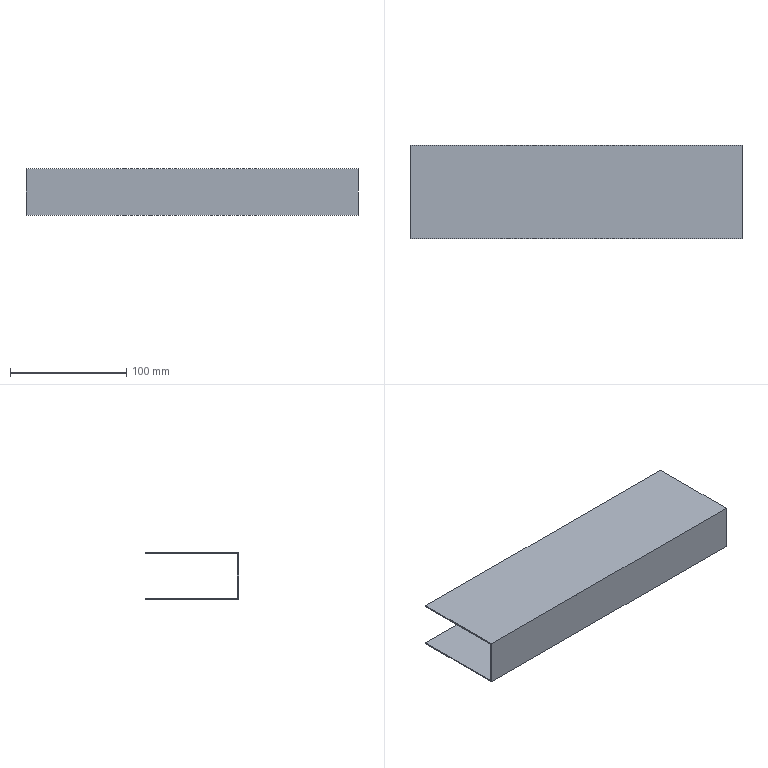Part | SolidWorks | features BaseBody 1 | 1 solid | 10 faces | box 285 x 80 x 40 mm | volume 56430 mm3 | plane 10
STEP:
#1=CARTESIAN_POINT('',(0.,1.,19.));
#2=VERTEX_POINT('',#1);
#3=CARTESIAN_POINT('',(0.,80.,19.));
#4=VERTEX_POINT('',#3);
#5=CARTESIAN_POINT('',(0.,0.,19.));
#6=DIRECTION('',(0.,1.,0.));
#7=VECTOR('',#6,1000.);
#8=LINE('',#5,#7);
#9=EDGE_CURVE('',#2,#4,#8,.T.);
#10=ORIENTED_EDGE('',*,*,#9,.F.);
#11=CARTESIAN_POINT('',(0.,1.,-19.));
#12=VERTEX_POINT('',#11);
#13=CARTESIAN_POINT('',(0.,1.,20.));
#14=DIRECTION('',(0.,0.,1.));
#15=VECTOR('',#14,1000.);
#16=LINE('',#13,#15);
#17=EDGE_CURVE('',#12,#2,#16,.T.);
#18=ORIENTED_EDGE('',*,*,#17,.F.);
#19=CARTESIAN_POINT('',(0.,80.,-19.));
#20=VERTEX_POINT('',#19);
#21=CARTESIAN_POINT('',(0.,0.,-19.));
#22=DIRECTION('',(0.,-1.,0.));
#23=VECTOR('',#22,1000.);
#24=LINE('',#21,#23);
#25=EDGE_CURVE('',#20,#12,#24,.T.);
#26=ORIENTED_EDGE('',*,*,#25,.F.);
#27=CARTESIAN_POINT('',(0.,80.,-20.));
#28=VERTEX_POINT('',#27);
#29=CARTESIAN_POINT('',(0.,80.,-19.));
#30=DIRECTION('',(0.,0.,-1.));
#31=VECTOR('',#30,1000.);
#32=LINE('',#29,#31);
#33=EDGE_CURVE('',#20,#28,#32,.T.);
#34=ORIENTED_EDGE('',*,*,#33,.T.);
#35=CARTESIAN_POINT('',(0.,0.,-20.));
#36=VERTEX_POINT('',#35);
#37=CARTESIAN_POINT('',(0.,0.,-20.));
#38=DIRECTION('',(0.,-1.,0.));
#39=VECTOR('',#38,1000.);
#40=LINE('',#37,#39);
#41=EDGE_CURVE('',#28,#36,#40,.T.);
#42=ORIENTED_EDGE('',*,*,#41,.T.);
#43=CARTESIAN_POINT('',(0.,0.,20.));
#44=VERTEX_POINT('',#43);
#45=CARTESIAN_POINT('',(0.,0.,20.));
#46=DIRECTION('',(0.,0.,1.));
#47=VECTOR('',#46,1000.);
#48=LINE('',#45,#47);
#49=EDGE_CURVE('',#36,#44,#48,.T.);
#50=ORIENTED_EDGE('',*,*,#49,.T.);
#51=CARTESIAN_POINT('',(0.,80.,20.));
#52=VERTEX_POINT('',#51);
#53=CARTESIAN_POINT('',(0.,0.,20.));
#54=DIRECTION('',(0.,1.,0.));
#55=VECTOR('',#54,1000.);
#56=LINE('',#53,#55);
#57=EDGE_CURVE('',#44,#52,#56,.T.);
#58=ORIENTED_EDGE('',*,*,#57,.T.);
#59=CARTESIAN_POINT('',(0.,80.,20.));
#60=DIRECTION('',(0.,0.,-1.));
#61=VECTOR('',#60,1000.);
#62=LINE('',#59,#61);
#63=EDGE_CURVE('',#52,#4,#62,.T.);
#64=ORIENTED_EDGE('',*,*,#63,.T.);
#65=EDGE_LOOP('',(#10,#18,#26,#34,#42,#50,#58,#64));
#66=FACE_OUTER_BOUND('',#65,.T.);
#67=CARTESIAN_POINT('',(0.,0.,0.));
#68=DIRECTION('',(-1.,0.,0.));
#69=DIRECTION('',(0.,0.,1.));
#70=AXIS2_PLACEMENT_3D('',#67,#68,#69);
#71=PLANE('',#70);
#72=ADVANCED_FACE('',(#66),#71,.T.);
#73=CARTESIAN_POINT('',(285.,1.,19.));
#74=VERTEX_POINT('',#73);
#75=CARTESIAN_POINT('',(285.,80.,19.));
#76=VERTEX_POINT('',#75);
#77=CARTESIAN_POINT('',(285.,0.,19.));
#78=DIRECTION('',(0.,1.,0.));
#79=VECTOR('',#78,1000.);
#80=LINE('',#77,#79);
#81=EDGE_CURVE('',#74,#76,#80,.T.);
#82=ORIENTED_EDGE('',*,*,#81,.T.);
#83=CARTESIAN_POINT('',(285.,80.,20.));
#84=VERTEX_POINT('',#83);
#85=CARTESIAN_POINT('',(285.,80.,20.));
#86=DIRECTION('',(0.,0.,-1.));
#87=VECTOR('',#86,1000.);
#88=LINE('',#85,#87);
#89=EDGE_CURVE('',#84,#76,#88,.T.);
#90=ORIENTED_EDGE('',*,*,#89,.F.);
#91=CARTESIAN_POINT('',(285.,0.,20.));
#92=VERTEX_POINT('',#91);
#93=CARTESIAN_POINT('',(285.,0.,20.));
#94=DIRECTION('',(0.,1.,0.));
#95=VECTOR('',#94,1000.);
#96=LINE('',#93,#95);
#97=EDGE_CURVE('',#92,#84,#96,.T.);
#98=ORIENTED_EDGE('',*,*,#97,.F.);
#99=CARTESIAN_POINT('',(285.,0.,-20.));
#100=VERTEX_POINT('',#99);
#101=CARTESIAN_POINT('',(285.,0.,20.));
#102=DIRECTION('',(0.,0.,1.));
#103=VECTOR('',#102,1000.);
#104=LINE('',#101,#103);
#105=EDGE_CURVE('',#100,#92,#104,.T.);
#106=ORIENTED_EDGE('',*,*,#105,.F.);
#107=CARTESIAN_POINT('',(285.,80.,-20.));
#108=VERTEX_POINT('',#107);
#109=CARTESIAN_POINT('',(285.,0.,-20.));
#110=DIRECTION('',(0.,-1.,0.));
#111=VECTOR('',#110,1000.);
#112=LINE('',#109,#111);
#113=EDGE_CURVE('',#108,#100,#112,.T.);
#114=ORIENTED_EDGE('',*,*,#113,.F.);
#115=CARTESIAN_POINT('',(285.,80.,-19.));
#116=VERTEX_POINT('',#115);
#117=CARTESIAN_POINT('',(285.,80.,-19.));
#118=DIRECTION('',(0.,0.,-1.));
#119=VECTOR('',#118,1000.);
#120=LINE('',#117,#119);
#121=EDGE_CURVE('',#116,#108,#120,.T.);
#122=ORIENTED_EDGE('',*,*,#121,.F.);
#123=CARTESIAN_POINT('',(285.,1.,-19.));
#124=VERTEX_POINT('',#123);
#125=CARTESIAN_POINT('',(285.,0.,-19.));
#126=DIRECTION('',(0.,-1.,0.));
#127=VECTOR('',#126,1000.);
#128=LINE('',#125,#127);
#129=EDGE_CURVE('',#116,#124,#128,.T.);
#130=ORIENTED_EDGE('',*,*,#129,.T.);
#131=CARTESIAN_POINT('',(285.,1.,20.));
#132=DIRECTION('',(0.,0.,1.));
#133=VECTOR('',#132,1000.);
#134=LINE('',#131,#133);
#135=EDGE_CURVE('',#124,#74,#134,.T.);
#136=ORIENTED_EDGE('',*,*,#135,.T.);
#137=EDGE_LOOP('',(#82,#90,#98,#106,#114,#122,#130,#136));
#138=FACE_OUTER_BOUND('',#137,.T.);
#139=CARTESIAN_POINT('',(285.,0.,0.));
#140=DIRECTION('',(-1.,0.,0.));
#141=DIRECTION('',(0.,0.,1.));
#142=AXIS2_PLACEMENT_3D('',#139,#140,#141);
#143=PLANE('',#142);
#144=ADVANCED_FACE('',(#138),#143,.F.);
#145=ORIENTED_EDGE('',*,*,#17,.T.);
#146=CARTESIAN_POINT('',(285.,1.,19.));
#147=DIRECTION('',(-1.,0.,0.));
#148=VECTOR('',#147,1000.);
#149=LINE('',#146,#148);
#150=EDGE_CURVE('',#74,#2,#149,.T.);
#151=ORIENTED_EDGE('',*,*,#150,.F.);
#152=ORIENTED_EDGE('',*,*,#135,.F.);
#153=CARTESIAN_POINT('',(285.,1.,-19.));
#154=DIRECTION('',(-1.,0.,0.));
#155=VECTOR('',#154,1000.);
#156=LINE('',#153,#155);
#157=EDGE_CURVE('',#124,#12,#156,.T.);
#158=ORIENTED_EDGE('',*,*,#157,.T.);
#159=EDGE_LOOP('',(#145,#151,#152,#158));
#160=FACE_OUTER_BOUND('',#159,.T.);
#161=CARTESIAN_POINT('',(285.,1.,20.));
#162=DIRECTION('',(0.,-1.,0.));
#163=DIRECTION('',(0.,0.,-1.));
#164=AXIS2_PLACEMENT_3D('',#161,#162,#163);
#165=PLANE('',#164);
#166=ADVANCED_FACE('',(#160),#165,.F.);
#167=ORIENTED_EDGE('',*,*,#25,.T.);
#168=ORIENTED_EDGE('',*,*,#157,.F.);
#169=ORIENTED_EDGE('',*,*,#129,.F.);
#170=CARTESIAN_POINT('',(285.,80.,-19.));
#171=DIRECTION('',(-1.,0.,0.));
#172=VECTOR('',#171,1000.);
#173=LINE('',#170,#172);
#174=EDGE_CURVE('',#116,#20,#173,.T.);
#175=ORIENTED_EDGE('',*,*,#174,.T.);
#176=EDGE_LOOP('',(#167,#168,#169,#175));
#177=FACE_OUTER_BOUND('',#176,.T.);
#178=CARTESIAN_POINT('',(285.,0.,-19.));
#179=DIRECTION('',(0.,0.,-1.));
#180=DIRECTION('',(0.,-1.,0.));
#181=AXIS2_PLACEMENT_3D('',#178,#179,#180);
#182=PLANE('',#181);
#183=ADVANCED_FACE('',(#177),#182,.F.);
#184=ORIENTED_EDGE('',*,*,#33,.F.);
#185=ORIENTED_EDGE('',*,*,#174,.F.);
#186=ORIENTED_EDGE('',*,*,#121,.T.);
#187=CARTESIAN_POINT('',(285.,80.,-20.));
#188=DIRECTION('',(-1.,0.,0.));
#189=VECTOR('',#188,1000.);
#190=LINE('',#187,#189);
#191=EDGE_CURVE('',#108,#28,#190,.T.);
#192=ORIENTED_EDGE('',*,*,#191,.T.);
#193=EDGE_LOOP('',(#184,#185,#186,#192));
#194=FACE_OUTER_BOUND('',#193,.T.);
#195=CARTESIAN_POINT('',(285.,80.,-19.));
#196=DIRECTION('',(0.,1.,0.));
#197=DIRECTION('',(1.,0.,0.));
#198=AXIS2_PLACEMENT_3D('',#195,#196,#197);
#199=PLANE('',#198);
#200=ADVANCED_FACE('',(#194),#199,.T.);
#201=ORIENTED_EDGE('',*,*,#41,.F.);
#202=ORIENTED_EDGE('',*,*,#191,.F.);
#203=ORIENTED_EDGE('',*,*,#113,.T.);
#204=CARTESIAN_POINT('',(285.,0.,-20.));
#205=DIRECTION('',(-1.,0.,0.));
#206=VECTOR('',#205,1000.);
#207=LINE('',#204,#206);
#208=EDGE_CURVE('',#100,#36,#207,.T.);
#209=ORIENTED_EDGE('',*,*,#208,.T.);
#210=EDGE_LOOP('',(#201,#202,#203,#209));
#211=FACE_OUTER_BOUND('',#210,.T.);
#212=CARTESIAN_POINT('',(285.,0.,-20.));
#213=DIRECTION('',(0.,0.,-1.));
#214=DIRECTION('',(0.,-1.,0.));
#215=AXIS2_PLACEMENT_3D('',#212,#213,#214);
#216=PLANE('',#215);
#217=ADVANCED_FACE('',(#211),#216,.T.);
#218=ORIENTED_EDGE('',*,*,#49,.F.);
#219=ORIENTED_EDGE('',*,*,#208,.F.);
#220=ORIENTED_EDGE('',*,*,#105,.T.);
#221=CARTESIAN_POINT('',(285.,0.,20.));
#222=DIRECTION('',(-1.,0.,0.));
#223=VECTOR('',#222,1000.);
#224=LINE('',#221,#223);
#225=EDGE_CURVE('',#92,#44,#224,.T.);
#226=ORIENTED_EDGE('',*,*,#225,.T.);
#227=EDGE_LOOP('',(#218,#219,#220,#226));
#228=FACE_OUTER_BOUND('',#227,.T.);
#229=CARTESIAN_POINT('',(285.,0.,20.));
#230=DIRECTION('',(0.,-1.,0.));
#231=DIRECTION('',(0.,0.,-1.));
#232=AXIS2_PLACEMENT_3D('',#229,#230,#231);
#233=PLANE('',#232);
#234=ADVANCED_FACE('',(#228),#233,.T.);
#235=ORIENTED_EDGE('',*,*,#57,.F.);
#236=ORIENTED_EDGE('',*,*,#225,.F.);
#237=ORIENTED_EDGE('',*,*,#97,.T.);
#238=CARTESIAN_POINT('',(285.,80.,20.));
#239=DIRECTION('',(-1.,0.,0.));
#240=VECTOR('',#239,1000.);
#241=LINE('',#238,#240);
#242=EDGE_CURVE('',#84,#52,#241,.T.);
#243=ORIENTED_EDGE('',*,*,#242,.T.);
#244=EDGE_LOOP('',(#235,#236,#237,#243));
#245=FACE_OUTER_BOUND('',#244,.T.);
#246=CARTESIAN_POINT('',(285.,0.,20.));
#247=DIRECTION('',(0.,0.,1.));
#248=DIRECTION('',(0.,-1.,0.));
#249=AXIS2_PLACEMENT_3D('',#246,#247,#248);
#250=PLANE('',#249);
#251=ADVANCED_FACE('',(#245),#250,.T.);
#252=ORIENTED_EDGE('',*,*,#63,.F.);
#253=ORIENTED_EDGE('',*,*,#242,.F.);
#254=ORIENTED_EDGE('',*,*,#89,.T.);
#255=CARTESIAN_POINT('',(285.,80.,19.));
#256=DIRECTION('',(-1.,0.,0.));
#257=VECTOR('',#256,1000.);
#258=LINE('',#255,#257);
#259=EDGE_CURVE('',#76,#4,#258,.T.);
#260=ORIENTED_EDGE('',*,*,#259,.T.);
#261=EDGE_LOOP('',(#252,#253,#254,#260));
#262=FACE_OUTER_BOUND('',#261,.T.);
#263=CARTESIAN_POINT('',(285.,80.,20.));
#264=DIRECTION('',(0.,1.,0.));
#265=DIRECTION('',(1.,0.,0.));
#266=AXIS2_PLACEMENT_3D('',#263,#264,#265);
#267=PLANE('',#266);
#268=ADVANCED_FACE('',(#262),#267,.T.);
#269=ORIENTED_EDGE('',*,*,#9,.T.);
#270=ORIENTED_EDGE('',*,*,#259,.F.);
#271=ORIENTED_EDGE('',*,*,#81,.F.);
#272=ORIENTED_EDGE('',*,*,#150,.T.);
#273=EDGE_LOOP('',(#269,#270,#271,#272));
#274=FACE_OUTER_BOUND('',#273,.T.);
#275=CARTESIAN_POINT('',(285.,0.,19.));
#276=DIRECTION('',(0.,0.,1.));
#277=DIRECTION('',(0.,-1.,0.));
#278=AXIS2_PLACEMENT_3D('',#275,#276,#277);
#279=PLANE('',#278);
#280=ADVANCED_FACE('',(#274),#279,.F.);
#281=CLOSED_SHELL('',(#72,#144,#166,#183,#200,#217,#234,#251,#268,#280));
#282=MANIFOLD_SOLID_BREP('',#281);
#283=CARTESIAN_POINT('',(0.,0.,0.));
#284=DIRECTION('',(0.,0.,1.));
#285=DIRECTION('',(1.,0.,0.));
#286=AXIS2_PLACEMENT_3D('',#283,#284,#285);
#287=(LENGTH_UNIT()NAMED_UNIT(*)SI_UNIT(.MILLI.,.METRE.));
#288=UNCERTAINTY_MEASURE_WITH_UNIT(LENGTH_MEASURE(0.00001),#287,'','');
#289=(NAMED_UNIT(*)PLANE_ANGLE_UNIT()SI_UNIT($,.RADIAN.));
#290=(NAMED_UNIT(*)SI_UNIT($,.STERADIAN.)SOLID_ANGLE_UNIT());
#291=(GEOMETRIC_REPRESENTATION_CONTEXT(3)GLOBAL_UNCERTAINTY_ASSIGNED_CONTEXT((#288))GLOBAL_UNIT_ASSIGNED_CONTEXT((#287,#289,#290))REPRESENTATION_CONTEXT('',''));
#292=ADVANCED_BREP_SHAPE_REPRESENTATION('',(#282,#286),#291);